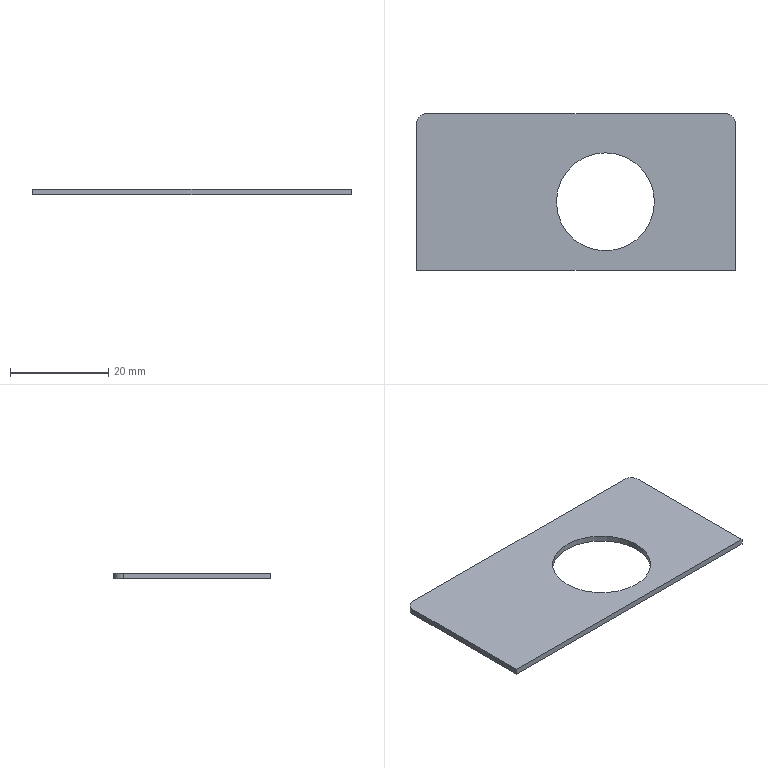Part | 1 solid | 10 faces | box 65 x 32 x 1.2 mm | volume 2117 mm3 | plane 6 | cylinder 4 | commonest cylinder face diameters 4 x2 20 x2
STEP:
#1=CARTESIAN_POINT('',(28.5,14.,0.));
#2=VERTEX_POINT('',#1);
#3=CARTESIAN_POINT('',(48.5,14.,0.));
#4=VERTEX_POINT('',#3);
#5=CARTESIAN_POINT('',(38.5,14.,0.));
#6=DIRECTION('',(0.,0.,1.));
#7=DIRECTION('',(1.,0.,0.));
#8=AXIS2_PLACEMENT_3D('',#5,#6,#7);
#9=CIRCLE('',#8,10.);
#10=EDGE_CURVE('',#2,#4,#9,.T.);
#11=ORIENTED_EDGE('',*,*,#10,.F.);
#12=CARTESIAN_POINT('',(28.5,14.,1.2));
#13=VERTEX_POINT('',#12);
#14=CARTESIAN_POINT('',(28.5,14.,0.));
#15=DIRECTION('',(0.,0.,1.));
#16=VECTOR('',#15,1000.);
#17=LINE('',#14,#16);
#18=EDGE_CURVE('',#2,#13,#17,.T.);
#19=ORIENTED_EDGE('',*,*,#18,.T.);
#20=CARTESIAN_POINT('',(48.5,14.,1.2));
#21=VERTEX_POINT('',#20);
#22=CARTESIAN_POINT('',(38.5,14.,1.2));
#23=DIRECTION('',(0.,0.,1.));
#24=DIRECTION('',(1.,0.,0.));
#25=AXIS2_PLACEMENT_3D('',#22,#23,#24);
#26=CIRCLE('',#25,10.);
#27=EDGE_CURVE('',#13,#21,#26,.T.);
#28=ORIENTED_EDGE('',*,*,#27,.T.);
#29=CARTESIAN_POINT('',(48.5,14.,0.));
#30=DIRECTION('',(0.,0.,1.));
#31=VECTOR('',#30,1000.);
#32=LINE('',#29,#31);
#33=EDGE_CURVE('',#4,#21,#32,.T.);
#34=ORIENTED_EDGE('',*,*,#33,.F.);
#35=EDGE_LOOP('',(#11,#19,#28,#34));
#36=FACE_OUTER_BOUND('',#35,.T.);
#37=CARTESIAN_POINT('',(38.5,14.,0.));
#38=DIRECTION('',(0.,0.,1.));
#39=DIRECTION('',(1.,0.,0.));
#40=AXIS2_PLACEMENT_3D('',#37,#38,#39);
#41=CYLINDRICAL_SURFACE('',#40,10.);
#42=ADVANCED_FACE('',(#36),#41,.F.);
#43=CARTESIAN_POINT('',(0.,30.,1.2));
#44=VERTEX_POINT('',#43);
#45=CARTESIAN_POINT('',(0.,0.,1.2));
#46=VERTEX_POINT('',#45);
#47=CARTESIAN_POINT('',(0.,0.,1.2));
#48=DIRECTION('',(0.,-1.,0.));
#49=VECTOR('',#48,1000.);
#50=LINE('',#47,#49);
#51=EDGE_CURVE('',#44,#46,#50,.T.);
#52=ORIENTED_EDGE('',*,*,#51,.F.);
#53=CARTESIAN_POINT('',(0.,30.,0.));
#54=VERTEX_POINT('',#53);
#55=CARTESIAN_POINT('',(0.,30.,1.2));
#56=DIRECTION('',(0.,0.,-1.));
#57=VECTOR('',#56,1000.);
#58=LINE('',#55,#57);
#59=EDGE_CURVE('',#44,#54,#58,.T.);
#60=ORIENTED_EDGE('',*,*,#59,.T.);
#61=CARTESIAN_POINT('',(0.,0.,0.));
#62=VERTEX_POINT('',#61);
#63=CARTESIAN_POINT('',(0.,0.,0.));
#64=DIRECTION('',(0.,-1.,0.));
#65=VECTOR('',#64,1000.);
#66=LINE('',#63,#65);
#67=EDGE_CURVE('',#54,#62,#66,.T.);
#68=ORIENTED_EDGE('',*,*,#67,.T.);
#69=CARTESIAN_POINT('',(0.,0.,1.2));
#70=DIRECTION('',(0.,0.,-1.));
#71=VECTOR('',#70,1000.);
#72=LINE('',#69,#71);
#73=EDGE_CURVE('',#46,#62,#72,.T.);
#74=ORIENTED_EDGE('',*,*,#73,.F.);
#75=EDGE_LOOP('',(#52,#60,#68,#74));
#76=FACE_OUTER_BOUND('',#75,.T.);
#77=CARTESIAN_POINT('',(0.,0.,1.2));
#78=DIRECTION('',(1.,0.,0.));
#79=DIRECTION('',(0.,0.,-1.));
#80=AXIS2_PLACEMENT_3D('',#77,#78,#79);
#81=PLANE('',#80);
#82=ADVANCED_FACE('',(#76),#81,.F.);
#83=CARTESIAN_POINT('',(65.,0.,0.));
#84=VERTEX_POINT('',#83);
#85=CARTESIAN_POINT('',(0.,0.,0.));
#86=DIRECTION('',(1.,0.,0.));
#87=VECTOR('',#86,1000.);
#88=LINE('',#85,#87);
#89=EDGE_CURVE('',#62,#84,#88,.T.);
#90=ORIENTED_EDGE('',*,*,#89,.T.);
#91=CARTESIAN_POINT('',(65.,0.,1.2));
#92=VERTEX_POINT('',#91);
#93=CARTESIAN_POINT('',(65.,0.,1.2));
#94=DIRECTION('',(0.,0.,-1.));
#95=VECTOR('',#94,1000.);
#96=LINE('',#93,#95);
#97=EDGE_CURVE('',#92,#84,#96,.T.);
#98=ORIENTED_EDGE('',*,*,#97,.F.);
#99=CARTESIAN_POINT('',(0.,0.,1.2));
#100=DIRECTION('',(1.,0.,0.));
#101=VECTOR('',#100,1000.);
#102=LINE('',#99,#101);
#103=EDGE_CURVE('',#46,#92,#102,.T.);
#104=ORIENTED_EDGE('',*,*,#103,.F.);
#105=ORIENTED_EDGE('',*,*,#73,.T.);
#106=EDGE_LOOP('',(#90,#98,#104,#105));
#107=FACE_OUTER_BOUND('',#106,.T.);
#108=CARTESIAN_POINT('',(0.,0.,1.2));
#109=DIRECTION('',(0.,1.,0.));
#110=DIRECTION('',(0.,0.,1.));
#111=AXIS2_PLACEMENT_3D('',#108,#109,#110);
#112=PLANE('',#111);
#113=ADVANCED_FACE('',(#107),#112,.F.);
#114=CARTESIAN_POINT('',(65.,30.,0.));
#115=VERTEX_POINT('',#114);
#116=CARTESIAN_POINT('',(65.,0.,0.));
#117=DIRECTION('',(0.,1.,0.));
#118=VECTOR('',#117,1000.);
#119=LINE('',#116,#118);
#120=EDGE_CURVE('',#84,#115,#119,.T.);
#121=ORIENTED_EDGE('',*,*,#120,.T.);
#122=CARTESIAN_POINT('',(65.,30.,1.2));
#123=VERTEX_POINT('',#122);
#124=CARTESIAN_POINT('',(65.,30.,1.2));
#125=DIRECTION('',(0.,0.,1.));
#126=VECTOR('',#125,1000.);
#127=LINE('',#124,#126);
#128=EDGE_CURVE('',#115,#123,#127,.T.);
#129=ORIENTED_EDGE('',*,*,#128,.T.);
#130=CARTESIAN_POINT('',(65.,0.,1.2));
#131=DIRECTION('',(0.,1.,0.));
#132=VECTOR('',#131,1000.);
#133=LINE('',#130,#132);
#134=EDGE_CURVE('',#92,#123,#133,.T.);
#135=ORIENTED_EDGE('',*,*,#134,.F.);
#136=ORIENTED_EDGE('',*,*,#97,.T.);
#137=EDGE_LOOP('',(#121,#129,#135,#136));
#138=FACE_OUTER_BOUND('',#137,.T.);
#139=CARTESIAN_POINT('',(65.,0.,1.2));
#140=DIRECTION('',(-1.,0.,0.));
#141=DIRECTION('',(0.,0.,1.));
#142=AXIS2_PLACEMENT_3D('',#139,#140,#141);
#143=PLANE('',#142);
#144=ADVANCED_FACE('',(#138),#143,.F.);
#145=CARTESIAN_POINT('',(63.,32.,0.));
#146=VERTEX_POINT('',#145);
#147=CARTESIAN_POINT('',(2.,32.,0.));
#148=VERTEX_POINT('',#147);
#149=CARTESIAN_POINT('',(0.,32.,0.));
#150=DIRECTION('',(-1.,0.,0.));
#151=VECTOR('',#150,1000.);
#152=LINE('',#149,#151);
#153=EDGE_CURVE('',#146,#148,#152,.T.);
#154=ORIENTED_EDGE('',*,*,#153,.T.);
#155=CARTESIAN_POINT('',(2.,32.,1.2));
#156=VERTEX_POINT('',#155);
#157=CARTESIAN_POINT('',(2.,32.,1.2));
#158=DIRECTION('',(0.,0.,1.));
#159=VECTOR('',#158,1000.);
#160=LINE('',#157,#159);
#161=EDGE_CURVE('',#148,#156,#160,.T.);
#162=ORIENTED_EDGE('',*,*,#161,.T.);
#163=CARTESIAN_POINT('',(63.,32.,1.2));
#164=VERTEX_POINT('',#163);
#165=CARTESIAN_POINT('',(0.,32.,1.2));
#166=DIRECTION('',(-1.,0.,0.));
#167=VECTOR('',#166,1000.);
#168=LINE('',#165,#167);
#169=EDGE_CURVE('',#164,#156,#168,.T.);
#170=ORIENTED_EDGE('',*,*,#169,.F.);
#171=CARTESIAN_POINT('',(63.,32.,1.2));
#172=DIRECTION('',(0.,0.,-1.));
#173=VECTOR('',#172,1000.);
#174=LINE('',#171,#173);
#175=EDGE_CURVE('',#164,#146,#174,.T.);
#176=ORIENTED_EDGE('',*,*,#175,.T.);
#177=EDGE_LOOP('',(#154,#162,#170,#176));
#178=FACE_OUTER_BOUND('',#177,.T.);
#179=CARTESIAN_POINT('',(0.,32.,1.2));
#180=DIRECTION('',(0.,-1.,0.));
#181=DIRECTION('',(0.,0.,-1.));
#182=AXIS2_PLACEMENT_3D('',#179,#180,#181);
#183=PLANE('',#182);
#184=ADVANCED_FACE('',(#178),#183,.F.);
#185=CARTESIAN_POINT('',(38.5,14.,1.2));
#186=DIRECTION('',(0.,0.,1.));
#187=DIRECTION('',(1.,0.,0.));
#188=AXIS2_PLACEMENT_3D('',#185,#186,#187);
#189=CIRCLE('',#188,10.);
#190=EDGE_CURVE('',#21,#13,#189,.T.);
#191=ORIENTED_EDGE('',*,*,#190,.F.);
#192=ORIENTED_EDGE('',*,*,#27,.F.);
#193=EDGE_LOOP('',(#191,#192));
#194=FACE_BOUND('',#193,.T.);
#195=ORIENTED_EDGE('',*,*,#169,.T.);
#196=CARTESIAN_POINT('',(2.,30.,1.2));
#197=DIRECTION('',(0.,0.,1.));
#198=DIRECTION('',(-1.,0.,0.));
#199=AXIS2_PLACEMENT_3D('',#196,#197,#198);
#200=CIRCLE('',#199,2.);
#201=EDGE_CURVE('',#156,#44,#200,.T.);
#202=ORIENTED_EDGE('',*,*,#201,.T.);
#203=ORIENTED_EDGE('',*,*,#51,.T.);
#204=ORIENTED_EDGE('',*,*,#103,.T.);
#205=ORIENTED_EDGE('',*,*,#134,.T.);
#206=CARTESIAN_POINT('',(63.,30.,1.2));
#207=DIRECTION('',(0.,0.,1.));
#208=DIRECTION('',(-1.,0.,0.));
#209=AXIS2_PLACEMENT_3D('',#206,#207,#208);
#210=CIRCLE('',#209,2.);
#211=EDGE_CURVE('',#123,#164,#210,.T.);
#212=ORIENTED_EDGE('',*,*,#211,.T.);
#213=EDGE_LOOP('',(#195,#202,#203,#204,#205,#212));
#214=FACE_OUTER_BOUND('',#213,.T.);
#215=CARTESIAN_POINT('',(0.,0.,1.2));
#216=DIRECTION('',(0.,0.,-1.));
#217=DIRECTION('',(-1.,0.,0.));
#218=AXIS2_PLACEMENT_3D('',#215,#216,#217);
#219=PLANE('',#218);
#220=ADVANCED_FACE('',(#194,#214),#219,.F.);
#221=CARTESIAN_POINT('',(38.5,14.,0.));
#222=DIRECTION('',(0.,0.,1.));
#223=DIRECTION('',(1.,0.,0.));
#224=AXIS2_PLACEMENT_3D('',#221,#222,#223);
#225=CIRCLE('',#224,10.);
#226=EDGE_CURVE('',#4,#2,#225,.T.);
#227=ORIENTED_EDGE('',*,*,#226,.T.);
#228=ORIENTED_EDGE('',*,*,#10,.T.);
#229=EDGE_LOOP('',(#227,#228));
#230=FACE_BOUND('',#229,.T.);
#231=ORIENTED_EDGE('',*,*,#67,.F.);
#232=CARTESIAN_POINT('',(2.,30.,0.));
#233=DIRECTION('',(0.,0.,-1.));
#234=DIRECTION('',(-1.,0.,0.));
#235=AXIS2_PLACEMENT_3D('',#232,#233,#234);
#236=CIRCLE('',#235,2.);
#237=EDGE_CURVE('',#54,#148,#236,.T.);
#238=ORIENTED_EDGE('',*,*,#237,.T.);
#239=ORIENTED_EDGE('',*,*,#153,.F.);
#240=CARTESIAN_POINT('',(63.,30.,0.));
#241=DIRECTION('',(0.,0.,-1.));
#242=DIRECTION('',(-1.,0.,0.));
#243=AXIS2_PLACEMENT_3D('',#240,#241,#242);
#244=CIRCLE('',#243,2.);
#245=EDGE_CURVE('',#146,#115,#244,.T.);
#246=ORIENTED_EDGE('',*,*,#245,.T.);
#247=ORIENTED_EDGE('',*,*,#120,.F.);
#248=ORIENTED_EDGE('',*,*,#89,.F.);
#249=EDGE_LOOP('',(#231,#238,#239,#246,#247,#248));
#250=FACE_OUTER_BOUND('',#249,.T.);
#251=CARTESIAN_POINT('',(0.,0.,0.));
#252=DIRECTION('',(0.,0.,-1.));
#253=DIRECTION('',(-1.,0.,0.));
#254=AXIS2_PLACEMENT_3D('',#251,#252,#253);
#255=PLANE('',#254);
#256=ADVANCED_FACE('',(#230,#250),#255,.T.);
#257=ORIENTED_EDGE('',*,*,#18,.F.);
#258=ORIENTED_EDGE('',*,*,#226,.F.);
#259=ORIENTED_EDGE('',*,*,#33,.T.);
#260=ORIENTED_EDGE('',*,*,#190,.T.);
#261=EDGE_LOOP('',(#257,#258,#259,#260));
#262=FACE_OUTER_BOUND('',#261,.T.);
#263=CARTESIAN_POINT('',(38.5,14.,0.));
#264=DIRECTION('',(0.,0.,1.));
#265=DIRECTION('',(1.,0.,0.));
#266=AXIS2_PLACEMENT_3D('',#263,#264,#265);
#267=CYLINDRICAL_SURFACE('',#266,10.);
#268=ADVANCED_FACE('',(#262),#267,.F.);
#269=ORIENTED_EDGE('',*,*,#201,.F.);
#270=ORIENTED_EDGE('',*,*,#161,.F.);
#271=ORIENTED_EDGE('',*,*,#237,.F.);
#272=ORIENTED_EDGE('',*,*,#59,.F.);
#273=EDGE_LOOP('',(#269,#270,#271,#272));
#274=FACE_OUTER_BOUND('',#273,.T.);
#275=CARTESIAN_POINT('',(2.,30.,1.2));
#276=DIRECTION('',(0.,0.,-1.));
#277=DIRECTION('',(-1.,0.,0.));
#278=AXIS2_PLACEMENT_3D('',#275,#276,#277);
#279=CYLINDRICAL_SURFACE('',#278,2.);
#280=ADVANCED_FACE('',(#274),#279,.T.);
#281=ORIENTED_EDGE('',*,*,#211,.F.);
#282=ORIENTED_EDGE('',*,*,#128,.F.);
#283=ORIENTED_EDGE('',*,*,#245,.F.);
#284=ORIENTED_EDGE('',*,*,#175,.F.);
#285=EDGE_LOOP('',(#281,#282,#283,#284));
#286=FACE_OUTER_BOUND('',#285,.T.);
#287=CARTESIAN_POINT('',(63.,30.,1.2));
#288=DIRECTION('',(0.,0.,-1.));
#289=DIRECTION('',(-1.,0.,0.));
#290=AXIS2_PLACEMENT_3D('',#287,#288,#289);
#291=CYLINDRICAL_SURFACE('',#290,2.);
#292=ADVANCED_FACE('',(#286),#291,.T.);
#293=CLOSED_SHELL('',(#42,#82,#113,#144,#184,#220,#256,#268,#280,#292));
#294=MANIFOLD_SOLID_BREP('',#293);
#295=CARTESIAN_POINT('',(0.,0.,0.));
#296=DIRECTION('',(0.,0.,1.));
#297=DIRECTION('',(1.,0.,0.));
#298=AXIS2_PLACEMENT_3D('',#295,#296,#297);
#299=(LENGTH_UNIT()NAMED_UNIT(*)SI_UNIT(.MILLI.,.METRE.));
#300=UNCERTAINTY_MEASURE_WITH_UNIT(LENGTH_MEASURE(0.00001),#299,'','');
#301=(NAMED_UNIT(*)PLANE_ANGLE_UNIT()SI_UNIT($,.RADIAN.));
#302=(NAMED_UNIT(*)SI_UNIT($,.STERADIAN.)SOLID_ANGLE_UNIT());
#303=(GEOMETRIC_REPRESENTATION_CONTEXT(3)GLOBAL_UNCERTAINTY_ASSIGNED_CONTEXT((#300))GLOBAL_UNIT_ASSIGNED_CONTEXT((#299,#301,#302))REPRESENTATION_CONTEXT('',''));
#304=ADVANCED_BREP_SHAPE_REPRESENTATION('',(#294,#298),#303);